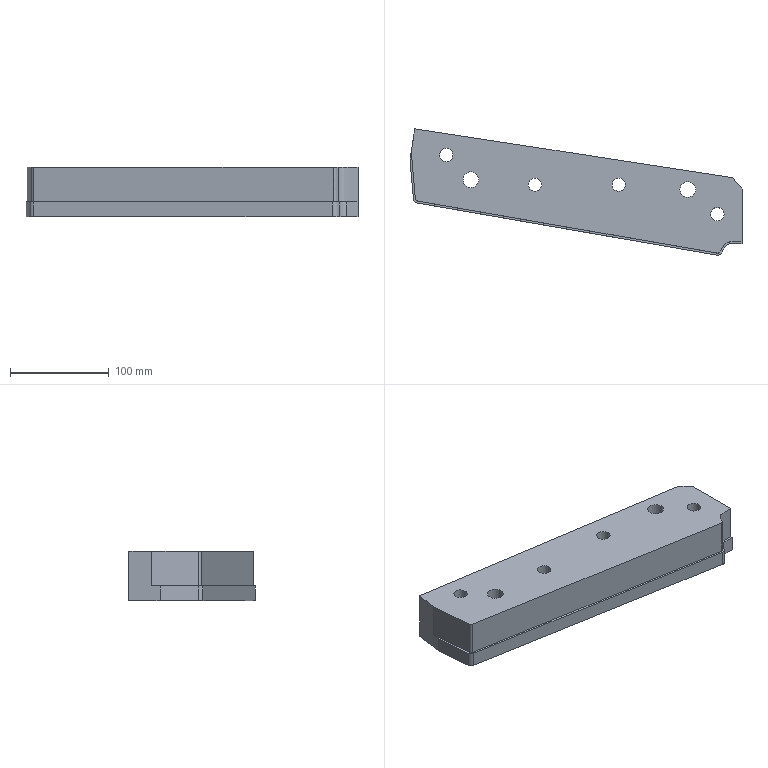Part | NX | features solid 2 | 1 solid | 40 faces | box 336.776 x 128.13 x 50 mm | volume 1036156 mm3 | plane 19 | cylinder 14 | spline 7 | commonest cylinder face diameters 13.5 x4 19.5 x4 16 x2 6 x1 10 x1 20 x1